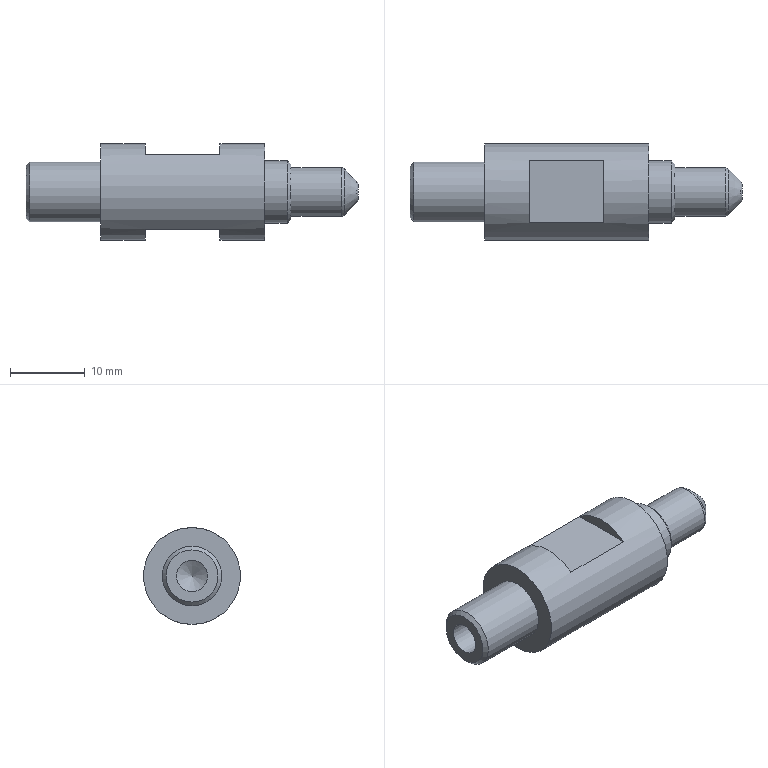Part | NX | features BREP 1 | 1 solid | 22 faces | box 44.5 x 13 x 13 mm | volume 3529 mm3 | plane 11 | cylinder 5 | cone 4 | torus 2 | commonest cylinder face diameters 4.2 x1 6.5 x1 8 x1 8.4 x1 13 x1
STEP:
#1=CARTESIAN_POINT('',(9.75,0.,-6.5));
#2=VERTEX_POINT('',#1);
#3=CARTESIAN_POINT('',(9.75,0.,0.));
#4=DIRECTION('',(1.,0.,0.));
#5=DIRECTION('',(0.,0.,-1.));
#6=AXIS2_PLACEMENT_3D('',#3,#4,#5);
#7=CIRCLE('',#6,6.5);
#8=EDGE_CURVE('',#2,#2,#7,.T.);
#9=ORIENTED_EDGE('',*,*,#8,.F.);
#10=EDGE_LOOP('',(#9));
#11=FACE_BOUND('',#10,.T.);
#12=CARTESIAN_POINT('',(-12.25,0.,-6.5));
#13=VERTEX_POINT('',#12);
#14=CARTESIAN_POINT('',(-12.25,0.,0.));
#15=DIRECTION('',(1.,0.,0.));
#16=DIRECTION('',(0.,0.,-1.));
#17=AXIS2_PLACEMENT_3D('',#14,#15,#16);
#18=CIRCLE('',#17,6.5);
#19=EDGE_CURVE('',#13,#13,#18,.T.);
#20=ORIENTED_EDGE('',*,*,#19,.T.);
#21=EDGE_LOOP('',(#20));
#22=FACE_BOUND('',#21,.T.);
#23=CARTESIAN_POINT('',(3.75,-4.153,-5.));
#24=VERTEX_POINT('',#23);
#25=CARTESIAN_POINT('',(-6.25,-4.153,-5.));
#26=VERTEX_POINT('',#25);
#27=CARTESIAN_POINT('',(-22.25,-4.153,-5.));
#28=DIRECTION('',(-1.,0.,0.));
#29=VECTOR('',#28,1000.);
#30=LINE('',#27,#29);
#31=EDGE_CURVE('',#24,#26,#30,.T.);
#32=ORIENTED_EDGE('',*,*,#31,.F.);
#33=CARTESIAN_POINT('',(3.75,4.153,-5.));
#34=VERTEX_POINT('',#33);
#35=CARTESIAN_POINT('',(3.75,0.,0.));
#36=DIRECTION('',(1.,0.,0.));
#37=DIRECTION('',(0.,0.,-1.));
#38=AXIS2_PLACEMENT_3D('',#35,#36,#37);
#39=CIRCLE('',#38,6.5);
#40=EDGE_CURVE('',#24,#34,#39,.T.);
#41=ORIENTED_EDGE('',*,*,#40,.T.);
#42=CARTESIAN_POINT('',(-6.25,4.153,-5.));
#43=VERTEX_POINT('',#42);
#44=CARTESIAN_POINT('',(-22.25,4.153,-5.));
#45=DIRECTION('',(1.,0.,0.));
#46=VECTOR('',#45,1000.);
#47=LINE('',#44,#46);
#48=EDGE_CURVE('',#43,#34,#47,.T.);
#49=ORIENTED_EDGE('',*,*,#48,.F.);
#50=CARTESIAN_POINT('',(-6.25,0.,0.));
#51=DIRECTION('',(1.,0.,0.));
#52=DIRECTION('',(0.,0.,-1.));
#53=AXIS2_PLACEMENT_3D('',#50,#51,#52);
#54=CIRCLE('',#53,6.5);
#55=EDGE_CURVE('',#26,#43,#54,.T.);
#56=ORIENTED_EDGE('',*,*,#55,.F.);
#57=EDGE_LOOP('',(#32,#41,#49,#56));
#58=FACE_BOUND('',#57,.T.);
#59=CARTESIAN_POINT('',(-6.25,-4.153,5.));
#60=VERTEX_POINT('',#59);
#61=CARTESIAN_POINT('',(-6.25,4.153,5.));
#62=VERTEX_POINT('',#61);
#63=CARTESIAN_POINT('',(-6.25,0.,0.));
#64=DIRECTION('',(-1.,0.,0.));
#65=DIRECTION('',(0.,0.,1.));
#66=AXIS2_PLACEMENT_3D('',#63,#64,#65);
#67=CIRCLE('',#66,6.5);
#68=EDGE_CURVE('',#60,#62,#67,.T.);
#69=ORIENTED_EDGE('',*,*,#68,.T.);
#70=CARTESIAN_POINT('',(3.75,4.153,5.));
#71=VERTEX_POINT('',#70);
#72=CARTESIAN_POINT('',(-22.25,4.153,5.));
#73=DIRECTION('',(-1.,0.,0.));
#74=VECTOR('',#73,1000.);
#75=LINE('',#72,#74);
#76=EDGE_CURVE('',#71,#62,#75,.T.);
#77=ORIENTED_EDGE('',*,*,#76,.F.);
#78=CARTESIAN_POINT('',(3.75,-4.153,5.));
#79=VERTEX_POINT('',#78);
#80=CARTESIAN_POINT('',(3.75,0.,0.));
#81=DIRECTION('',(-1.,0.,0.));
#82=DIRECTION('',(0.,0.,1.));
#83=AXIS2_PLACEMENT_3D('',#80,#81,#82);
#84=CIRCLE('',#83,6.5);
#85=EDGE_CURVE('',#79,#71,#84,.T.);
#86=ORIENTED_EDGE('',*,*,#85,.F.);
#87=CARTESIAN_POINT('',(-22.25,-4.153,5.));
#88=DIRECTION('',(1.,0.,0.));
#89=VECTOR('',#88,1000.);
#90=LINE('',#87,#89);
#91=EDGE_CURVE('',#60,#79,#90,.T.);
#92=ORIENTED_EDGE('',*,*,#91,.F.);
#93=EDGE_LOOP('',(#69,#77,#86,#92));
#94=FACE_BOUND('',#93,.T.);
#95=CARTESIAN_POINT('',(-22.25,0.,0.));
#96=DIRECTION('',(-1.,0.,0.));
#97=DIRECTION('',(0.,0.,1.));
#98=AXIS2_PLACEMENT_3D('',#95,#96,#97);
#99=CYLINDRICAL_SURFACE('',#98,6.5);
#100=ADVANCED_FACE('',(#11,#22,#58,#94),#99,.T.);
#101=CARTESIAN_POINT('',(-22.25,0.,3.5));
#102=VERTEX_POINT('',#101);
#103=CARTESIAN_POINT('',(-22.25,0.,0.));
#104=DIRECTION('',(1.,0.,0.));
#105=DIRECTION('',(0.,0.,1.));
#106=AXIS2_PLACEMENT_3D('',#103,#104,#105);
#107=CIRCLE('',#106,3.5);
#108=EDGE_CURVE('',#102,#102,#107,.T.);
#109=ORIENTED_EDGE('',*,*,#108,.F.);
#110=EDGE_LOOP('',(#109));
#111=FACE_BOUND('',#110,.T.);
#112=CARTESIAN_POINT('',(-22.25,0.,-2.1));
#113=VERTEX_POINT('',#112);
#114=CARTESIAN_POINT('',(-22.25,0.,0.));
#115=DIRECTION('',(1.,0.,0.));
#116=DIRECTION('',(0.,0.,-1.));
#117=AXIS2_PLACEMENT_3D('',#114,#115,#116);
#118=CIRCLE('',#117,2.1);
#119=EDGE_CURVE('',#113,#113,#118,.T.);
#120=ORIENTED_EDGE('',*,*,#119,.T.);
#121=EDGE_LOOP('',(#120));
#122=FACE_BOUND('',#121,.T.);
#123=CARTESIAN_POINT('',(-22.25,4.,0.));
#124=DIRECTION('',(1.,0.,0.));
#125=DIRECTION('',(0.,0.,-1.));
#126=AXIS2_PLACEMENT_3D('',#123,#124,#125);
#127=PLANE('',#126);
#128=ADVANCED_FACE('',(#111,#122),#127,.F.);
#129=CARTESIAN_POINT('',(22.25,0.,-1.043));
#130=VERTEX_POINT('',#129);
#131=CARTESIAN_POINT('',(22.25,0.,0.));
#132=DIRECTION('',(-1.,0.,0.));
#133=DIRECTION('',(0.,0.,-1.));
#134=AXIS2_PLACEMENT_3D('',#131,#132,#133);
#135=CIRCLE('',#134,1.043);
#136=EDGE_CURVE('',#130,#130,#135,.T.);
#137=ORIENTED_EDGE('',*,*,#136,.F.);
#138=EDGE_LOOP('',(#137));
#139=FACE_BOUND('',#138,.T.);
#140=CARTESIAN_POINT('',(22.25,0.,0.));
#141=DIRECTION('',(-1.,0.,0.));
#142=DIRECTION('',(0.,0.,1.));
#143=AXIS2_PLACEMENT_3D('',#140,#141,#142);
#144=PLANE('',#143);
#145=ADVANCED_FACE('',(#139),#144,.F.);
#146=CARTESIAN_POINT('',(20.043,0.,3.25));
#147=VERTEX_POINT('',#146);
#148=CARTESIAN_POINT('',(20.043,0.,0.));
#149=DIRECTION('',(1.,0.,0.));
#150=DIRECTION('',(0.,0.,1.));
#151=AXIS2_PLACEMENT_3D('',#148,#149,#150);
#152=CIRCLE('',#151,3.25);
#153=EDGE_CURVE('',#147,#147,#152,.T.);
#154=ORIENTED_EDGE('',*,*,#153,.F.);
#155=EDGE_LOOP('',(#154));
#156=FACE_BOUND('',#155,.T.);
#157=CARTESIAN_POINT('',(13.25,0.,-3.25));
#158=VERTEX_POINT('',#157);
#159=CARTESIAN_POINT('',(13.25,0.,0.));
#160=DIRECTION('',(1.,0.,0.));
#161=DIRECTION('',(0.,0.,-1.));
#162=AXIS2_PLACEMENT_3D('',#159,#160,#161);
#163=CIRCLE('',#162,3.25);
#164=EDGE_CURVE('',#158,#158,#163,.T.);
#165=ORIENTED_EDGE('',*,*,#164,.T.);
#166=EDGE_LOOP('',(#165));
#167=FACE_BOUND('',#166,.T.);
#168=CARTESIAN_POINT('',(-22.25,0.,0.));
#169=DIRECTION('',(-1.,0.,0.));
#170=DIRECTION('',(0.,0.,1.));
#171=AXIS2_PLACEMENT_3D('',#168,#169,#170);
#172=CYLINDRICAL_SURFACE('',#171,3.25);
#173=ADVANCED_FACE('',(#156,#167),#172,.T.);
#174=CARTESIAN_POINT('',(13.25,0.,-3.7));
#175=VERTEX_POINT('',#174);
#176=CARTESIAN_POINT('',(13.25,0.,0.));
#177=DIRECTION('',(-1.,0.,0.));
#178=DIRECTION('',(0.,0.,-1.));
#179=AXIS2_PLACEMENT_3D('',#176,#177,#178);
#180=CIRCLE('',#179,3.7);
#181=EDGE_CURVE('',#175,#175,#180,.T.);
#182=ORIENTED_EDGE('',*,*,#181,.F.);
#183=EDGE_LOOP('',(#182));
#184=FACE_BOUND('',#183,.T.);
#185=ORIENTED_EDGE('',*,*,#164,.F.);
#186=EDGE_LOOP('',(#185));
#187=FACE_BOUND('',#186,.T.);
#188=CARTESIAN_POINT('',(13.25,3.25,0.));
#189=DIRECTION('',(-1.,0.,0.));
#190=DIRECTION('',(0.,0.,1.));
#191=AXIS2_PLACEMENT_3D('',#188,#189,#190);
#192=PLANE('',#191);
#193=ADVANCED_FACE('',(#184,#187),#192,.F.);
#194=CARTESIAN_POINT('',(12.75,0.,-4.2));
#195=VERTEX_POINT('',#194);
#196=CARTESIAN_POINT('',(12.75,0.,0.));
#197=DIRECTION('',(1.,0.,0.));
#198=DIRECTION('',(0.,0.,-1.));
#199=AXIS2_PLACEMENT_3D('',#196,#197,#198);
#200=CIRCLE('',#199,4.2);
#201=EDGE_CURVE('',#195,#195,#200,.T.);
#202=ORIENTED_EDGE('',*,*,#201,.F.);
#203=EDGE_LOOP('',(#202));
#204=FACE_BOUND('',#203,.T.);
#205=CARTESIAN_POINT('',(9.75,0.,-4.2));
#206=VERTEX_POINT('',#205);
#207=CARTESIAN_POINT('',(9.75,0.,0.));
#208=DIRECTION('',(1.,0.,0.));
#209=DIRECTION('',(0.,0.,-1.));
#210=AXIS2_PLACEMENT_3D('',#207,#208,#209);
#211=CIRCLE('',#210,4.2);
#212=EDGE_CURVE('',#206,#206,#211,.T.);
#213=ORIENTED_EDGE('',*,*,#212,.T.);
#214=EDGE_LOOP('',(#213));
#215=FACE_BOUND('',#214,.T.);
#216=CARTESIAN_POINT('',(-22.25,0.,0.));
#217=DIRECTION('',(-1.,0.,0.));
#218=DIRECTION('',(0.,0.,1.));
#219=AXIS2_PLACEMENT_3D('',#216,#217,#218);
#220=CYLINDRICAL_SURFACE('',#219,4.2);
#221=ADVANCED_FACE('',(#204,#215),#220,.T.);
#222=ORIENTED_EDGE('',*,*,#8,.T.);
#223=EDGE_LOOP('',(#222));
#224=FACE_BOUND('',#223,.T.);
#225=ORIENTED_EDGE('',*,*,#212,.F.);
#226=EDGE_LOOP('',(#225));
#227=FACE_BOUND('',#226,.T.);
#228=CARTESIAN_POINT('',(9.75,4.2,0.));
#229=DIRECTION('',(-1.,0.,0.));
#230=DIRECTION('',(0.,0.,1.));
#231=AXIS2_PLACEMENT_3D('',#228,#229,#230);
#232=PLANE('',#231);
#233=ADVANCED_FACE('',(#224,#227),#232,.F.);
#234=CARTESIAN_POINT('',(-12.25,0.,-4.));
#235=VERTEX_POINT('',#234);
#236=CARTESIAN_POINT('',(-12.25,0.,0.));
#237=DIRECTION('',(1.,0.,0.));
#238=DIRECTION('',(0.,0.,-1.));
#239=AXIS2_PLACEMENT_3D('',#236,#237,#238);
#240=CIRCLE('',#239,4.);
#241=EDGE_CURVE('',#235,#235,#240,.T.);
#242=ORIENTED_EDGE('',*,*,#241,.T.);
#243=EDGE_LOOP('',(#242));
#244=FACE_BOUND('',#243,.T.);
#245=ORIENTED_EDGE('',*,*,#19,.F.);
#246=EDGE_LOOP('',(#245));
#247=FACE_BOUND('',#246,.T.);
#248=CARTESIAN_POINT('',(-12.25,6.5,0.));
#249=DIRECTION('',(1.,0.,0.));
#250=DIRECTION('',(0.,0.,-1.));
#251=AXIS2_PLACEMENT_3D('',#248,#249,#250);
#252=PLANE('',#251);
#253=ADVANCED_FACE('',(#244,#247),#252,.F.);
#254=CARTESIAN_POINT('',(-21.75,0.,4.));
#255=VERTEX_POINT('',#254);
#256=CARTESIAN_POINT('',(-21.75,0.,0.));
#257=DIRECTION('',(-1.,0.,0.));
#258=DIRECTION('',(0.,0.,1.));
#259=AXIS2_PLACEMENT_3D('',#256,#257,#258);
#260=CIRCLE('',#259,4.);
#261=EDGE_CURVE('',#255,#255,#260,.T.);
#262=ORIENTED_EDGE('',*,*,#261,.F.);
#263=EDGE_LOOP('',(#262));
#264=FACE_BOUND('',#263,.T.);
#265=ORIENTED_EDGE('',*,*,#241,.F.);
#266=EDGE_LOOP('',(#265));
#267=FACE_BOUND('',#266,.T.);
#268=CARTESIAN_POINT('',(-22.25,0.,0.));
#269=DIRECTION('',(-1.,0.,0.));
#270=DIRECTION('',(0.,0.,1.));
#271=AXIS2_PLACEMENT_3D('',#268,#269,#270);
#272=CYLINDRICAL_SURFACE('',#271,4.);
#273=ADVANCED_FACE('',(#264,#267),#272,.T.);
#274=CARTESIAN_POINT('',(22.104,0.,-1.396));
#275=VERTEX_POINT('',#274);
#276=CARTESIAN_POINT('',(22.104,0.,0.));
#277=DIRECTION('',(1.,0.,0.));
#278=DIRECTION('',(0.,0.,-1.));
#279=AXIS2_PLACEMENT_3D('',#276,#277,#278);
#280=CIRCLE('',#279,1.396);
#281=EDGE_CURVE('',#275,#275,#280,.T.);
#282=ORIENTED_EDGE('',*,*,#281,.F.);
#283=EDGE_LOOP('',(#282));
#284=FACE_BOUND('',#283,.T.);
#285=CARTESIAN_POINT('',(20.396,0.,-3.104));
#286=VERTEX_POINT('',#285);
#287=CARTESIAN_POINT('',(20.396,0.,0.));
#288=DIRECTION('',(-1.,0.,0.));
#289=DIRECTION('',(0.,0.,-1.));
#290=AXIS2_PLACEMENT_3D('',#287,#288,#289);
#291=CIRCLE('',#290,3.104);
#292=EDGE_CURVE('',#286,#286,#291,.T.);
#293=ORIENTED_EDGE('',*,*,#292,.F.);
#294=EDGE_LOOP('',(#293));
#295=FACE_BOUND('',#294,.T.);
#296=CARTESIAN_POINT('',(20.25,0.,0.));
#297=DIRECTION('',(-1.,0.,0.));
#298=DIRECTION('',(0.,0.,1.));
#299=AXIS2_PLACEMENT_3D('',#296,#297,#298);
#300=CONICAL_SURFACE('',#299,3.25,0.7854);
#301=ADVANCED_FACE('',(#284,#295),#300,.T.);
#302=ORIENTED_EDGE('',*,*,#181,.T.);
#303=EDGE_LOOP('',(#302));
#304=FACE_BOUND('',#303,.T.);
#305=ORIENTED_EDGE('',*,*,#201,.T.);
#306=EDGE_LOOP('',(#305));
#307=FACE_BOUND('',#306,.T.);
#308=CARTESIAN_POINT('',(12.75,0.,0.));
#309=DIRECTION('',(-1.,0.,0.));
#310=DIRECTION('',(0.,0.,1.));
#311=AXIS2_PLACEMENT_3D('',#308,#309,#310);
#312=CONICAL_SURFACE('',#311,4.2,0.7854);
#313=ADVANCED_FACE('',(#304,#307),#312,.T.);
#314=ORIENTED_EDGE('',*,*,#281,.T.);
#315=EDGE_LOOP('',(#314));
#316=FACE_BOUND('',#315,.T.);
#317=ORIENTED_EDGE('',*,*,#136,.T.);
#318=EDGE_LOOP('',(#317));
#319=FACE_BOUND('',#318,.T.);
#320=CARTESIAN_POINT('',(21.75,0.,0.));
#321=DIRECTION('',(-1.,0.,0.));
#322=DIRECTION('',(0.,0.,1.));
#323=AXIS2_PLACEMENT_3D('',#320,#321,#322);
#324=TOROIDAL_SURFACE('',#323,1.043,0.5);
#325=ADVANCED_FACE('',(#316,#319),#324,.T.);
#326=ORIENTED_EDGE('',*,*,#292,.T.);
#327=EDGE_LOOP('',(#326));
#328=FACE_BOUND('',#327,.T.);
#329=ORIENTED_EDGE('',*,*,#153,.T.);
#330=EDGE_LOOP('',(#329));
#331=FACE_BOUND('',#330,.T.);
#332=CARTESIAN_POINT('',(20.043,0.,0.));
#333=DIRECTION('',(1.,0.,0.));
#334=DIRECTION('',(0.,0.,-1.));
#335=AXIS2_PLACEMENT_3D('',#332,#333,#334);
#336=TOROIDAL_SURFACE('',#335,2.75,0.5);
#337=ADVANCED_FACE('',(#328,#331),#336,.T.);
#338=CARTESIAN_POINT('',(3.75,-7.887,-5.));
#339=DIRECTION('',(0.,1.,0.));
#340=VECTOR('',#339,1000.);
#341=LINE('',#338,#340);
#342=EDGE_CURVE('',#24,#34,#341,.T.);
#343=ORIENTED_EDGE('',*,*,#342,.F.);
#344=ORIENTED_EDGE('',*,*,#31,.T.);
#345=CARTESIAN_POINT('',(-6.25,-7.887,-5.));
#346=DIRECTION('',(0.,1.,0.));
#347=VECTOR('',#346,1000.);
#348=LINE('',#345,#347);
#349=EDGE_CURVE('',#26,#43,#348,.T.);
#350=ORIENTED_EDGE('',*,*,#349,.T.);
#351=ORIENTED_EDGE('',*,*,#48,.T.);
#352=EDGE_LOOP('',(#343,#344,#350,#351));
#353=FACE_BOUND('',#352,.T.);
#354=CARTESIAN_POINT('',(-6.25,-7.887,-5.));
#355=DIRECTION('',(0.,0.,1.));
#356=DIRECTION('',(1.,0.,0.));
#357=AXIS2_PLACEMENT_3D('',#354,#355,#356);
#358=PLANE('',#357);
#359=ADVANCED_FACE('',(#353),#358,.F.);
#360=ORIENTED_EDGE('',*,*,#349,.F.);
#361=ORIENTED_EDGE('',*,*,#55,.T.);
#362=EDGE_LOOP('',(#360,#361));
#363=FACE_BOUND('',#362,.T.);
#364=CARTESIAN_POINT('',(-6.25,0.,0.));
#365=DIRECTION('',(-1.,0.,0.));
#366=DIRECTION('',(0.,0.,1.));
#367=AXIS2_PLACEMENT_3D('',#364,#365,#366);
#368=PLANE('',#367);
#369=ADVANCED_FACE('',(#363),#368,.F.);
#370=ORIENTED_EDGE('',*,*,#40,.F.);
#371=ORIENTED_EDGE('',*,*,#342,.T.);
#372=EDGE_LOOP('',(#370,#371));
#373=FACE_BOUND('',#372,.T.);
#374=CARTESIAN_POINT('',(3.75,0.,0.));
#375=DIRECTION('',(-1.,0.,0.));
#376=DIRECTION('',(0.,0.,1.));
#377=AXIS2_PLACEMENT_3D('',#374,#375,#376);
#378=PLANE('',#377);
#379=ADVANCED_FACE('',(#373),#378,.T.);
#380=CARTESIAN_POINT('',(3.75,-7.887,5.));
#381=DIRECTION('',(0.,-1.,0.));
#382=VECTOR('',#381,1000.);
#383=LINE('',#380,#382);
#384=EDGE_CURVE('',#71,#79,#383,.T.);
#385=ORIENTED_EDGE('',*,*,#384,.F.);
#386=ORIENTED_EDGE('',*,*,#76,.T.);
#387=CARTESIAN_POINT('',(-6.25,-7.887,5.));
#388=DIRECTION('',(0.,-1.,0.));
#389=VECTOR('',#388,1000.);
#390=LINE('',#387,#389);
#391=EDGE_CURVE('',#62,#60,#390,.T.);
#392=ORIENTED_EDGE('',*,*,#391,.T.);
#393=ORIENTED_EDGE('',*,*,#91,.T.);
#394=EDGE_LOOP('',(#385,#386,#392,#393));
#395=FACE_BOUND('',#394,.T.);
#396=CARTESIAN_POINT('',(-6.25,-7.887,5.));
#397=DIRECTION('',(0.,0.,-1.));
#398=DIRECTION('',(-1.,0.,0.));
#399=AXIS2_PLACEMENT_3D('',#396,#397,#398);
#400=PLANE('',#399);
#401=ADVANCED_FACE('',(#395),#400,.F.);
#402=ORIENTED_EDGE('',*,*,#68,.F.);
#403=ORIENTED_EDGE('',*,*,#391,.F.);
#404=EDGE_LOOP('',(#402,#403));
#405=FACE_BOUND('',#404,.T.);
#406=CARTESIAN_POINT('',(-6.25,0.,0.));
#407=DIRECTION('',(1.,0.,0.));
#408=DIRECTION('',(0.,0.,-1.));
#409=AXIS2_PLACEMENT_3D('',#406,#407,#408);
#410=PLANE('',#409);
#411=ADVANCED_FACE('',(#405),#410,.T.);
#412=ORIENTED_EDGE('',*,*,#384,.T.);
#413=ORIENTED_EDGE('',*,*,#85,.T.);
#414=EDGE_LOOP('',(#412,#413));
#415=FACE_BOUND('',#414,.T.);
#416=CARTESIAN_POINT('',(3.75,0.,0.));
#417=DIRECTION('',(1.,0.,0.));
#418=DIRECTION('',(0.,0.,-1.));
#419=AXIS2_PLACEMENT_3D('',#416,#417,#418);
#420=PLANE('',#419);
#421=ADVANCED_FACE('',(#415),#420,.F.);
#422=CARTESIAN_POINT('',(-8.588,0.,0.));
#423=VERTEX_POINT('',#422);
#424=VERTEX_LOOP('',#423);
#425=FACE_BOUND('',#424,.T.);
#426=CARTESIAN_POINT('',(-9.85,0.,-2.1));
#427=VERTEX_POINT('',#426);
#428=CARTESIAN_POINT('',(-9.85,0.,0.));
#429=DIRECTION('',(1.,0.,0.));
#430=DIRECTION('',(0.,0.,-1.));
#431=AXIS2_PLACEMENT_3D('',#428,#429,#430);
#432=CIRCLE('',#431,2.1);
#433=EDGE_CURVE('',#427,#427,#432,.T.);
#434=ORIENTED_EDGE('',*,*,#433,.F.);
#435=EDGE_LOOP('',(#434));
#436=FACE_BOUND('',#435,.T.);
#437=CARTESIAN_POINT('',(-9.85,0.,0.));
#438=DIRECTION('',(-1.,0.,0.));
#439=DIRECTION('',(0.,0.,1.));
#440=AXIS2_PLACEMENT_3D('',#437,#438,#439);
#441=CONICAL_SURFACE('',#440,2.1,1.03);
#442=ADVANCED_FACE('',(#425,#436),#441,.F.);
#443=ORIENTED_EDGE('',*,*,#433,.T.);
#444=EDGE_LOOP('',(#443));
#445=FACE_BOUND('',#444,.T.);
#446=ORIENTED_EDGE('',*,*,#119,.F.);
#447=EDGE_LOOP('',(#446));
#448=FACE_BOUND('',#447,.T.);
#449=CARTESIAN_POINT('',(-22.25,0.,0.));
#450=DIRECTION('',(-1.,0.,0.));
#451=DIRECTION('',(0.,0.,1.));
#452=AXIS2_PLACEMENT_3D('',#449,#450,#451);
#453=CYLINDRICAL_SURFACE('',#452,2.1);
#454=ADVANCED_FACE('',(#445,#448),#453,.F.);
#455=ORIENTED_EDGE('',*,*,#261,.T.);
#456=EDGE_LOOP('',(#455));
#457=FACE_BOUND('',#456,.T.);
#458=ORIENTED_EDGE('',*,*,#108,.T.);
#459=EDGE_LOOP('',(#458));
#460=FACE_BOUND('',#459,.T.);
#461=CARTESIAN_POINT('',(-22.25,0.,0.));
#462=DIRECTION('',(1.,0.,0.));
#463=DIRECTION('',(0.,0.,-1.));
#464=AXIS2_PLACEMENT_3D('',#461,#462,#463);
#465=CONICAL_SURFACE('',#464,3.5,0.7854);
#466=ADVANCED_FACE('',(#457,#460),#465,.T.);
#467=CLOSED_SHELL('',(#100,#128,#145,#173,#193,#221,#233,#253,#273,#301,#313,#325,#337,#359,#369,#379,#401,#411,#421,#442,#454,#466));
#468=MANIFOLD_SOLID_BREP('',#467);
#469=(LENGTH_UNIT()NAMED_UNIT(*)SI_UNIT(.MILLI.,.METRE.));
#470=UNCERTAINTY_MEASURE_WITH_UNIT(LENGTH_MEASURE(0.00001),#469,'','');
#471=(NAMED_UNIT(*)PLANE_ANGLE_UNIT()SI_UNIT($,.RADIAN.));
#472=(NAMED_UNIT(*)SI_UNIT($,.STERADIAN.)SOLID_ANGLE_UNIT());
#473=(GEOMETRIC_REPRESENTATION_CONTEXT(3)GLOBAL_UNCERTAINTY_ASSIGNED_CONTEXT((#470))GLOBAL_UNIT_ASSIGNED_CONTEXT((#469,#471,#472))REPRESENTATION_CONTEXT('',''));
#474=ADVANCED_BREP_SHAPE_REPRESENTATION('',(#468),#473);